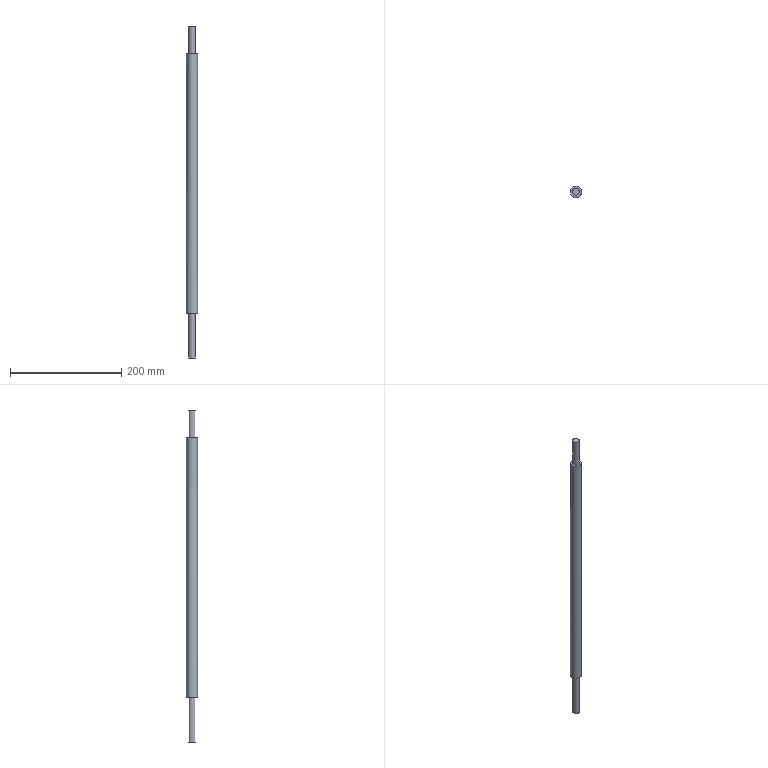Part | STEP file | chuandongzhou | 1 solid | 7 faces | box 20 x 20 x 596.6 mm | volume 161289 mm3 | plane 4 | cylinder 3 | commonest cylinder face diameters 12 x2 20 x1
STEP:
#1=CARTESIAN_POINT('',(0.,0.,0.));
#2=DIRECTION('',(0.,0.,1.));
#3=DIRECTION('',(1.,0.,0.));
#4=AXIS2_PLACEMENT_3D('',#1,#2,#3);
#5=CARTESIAN_POINT('',(-1061.818,-832.005,-786.336));
#6=VERTEX_POINT('',#5);
#7=CARTESIAN_POINT('',(-1061.818,-842.005,-786.336));
#8=DIRECTION('',(0.,0.,1.));
#9=DIRECTION('',(0.,1.,0.));
#10=AXIS2_PLACEMENT_3D('',#7,#8,#9);
#11=CIRCLE('',#10,10.);
#12=CARTESIAN_POINT('',(-1061.818,-842.005,-95.741));
#13=DIRECTION('',(0.,0.,-1.));
#14=DIRECTION('',(0.,1.,0.));
#15=AXIS2_PLACEMENT_3D('',#12,#13,#14);
#16=CYLINDRICAL_SURFACE('',#15,10.);
#17=CARTESIAN_POINT('',(6.283,690.595));
#18=DIRECTION('',(-1.,0.));
#19=VECTOR('',#18,1.);
#20=LINE('',#17,#19);
#21=(GEOMETRIC_REPRESENTATION_CONTEXT(2)PARAMETRIC_REPRESENTATION_CONTEXT()REPRESENTATION_CONTEXT('',''));
#22=DEFINITIONAL_REPRESENTATION('',(#20),#21);
#23=PCURVE('',#16,#22);
#24=CARTESIAN_POINT('',(-1061.818,-842.005,-786.336));
#25=DIRECTION('',(0.,0.,-1.));
#26=DIRECTION('',(0.,1.,0.));
#27=AXIS2_PLACEMENT_3D('',#24,#25,#26);
#28=PLANE('',#27);
#29=CARTESIAN_POINT('',(10.,0.));
#30=CARTESIAN_POINT('',(10.,-17.321));
#31=CARTESIAN_POINT('',(-5.,-8.66));
#32=CARTESIAN_POINT('',(-20.,0.));
#33=CARTESIAN_POINT('',(-5.,8.66));
#34=CARTESIAN_POINT('',(10.,17.321));
#35=CARTESIAN_POINT('',(10.,0.));
#36=(BOUNDED_CURVE()B_SPLINE_CURVE(2,(#29,#30,#31,#32,#33,#34,#35),.UNSPECIFIED.,.T.,.F.)B_SPLINE_CURVE_WITH_KNOTS((1,2,2,2,2,1),(-2.094,0.,2.094,4.189,6.283,8.378),.UNSPECIFIED.)CURVE()GEOMETRIC_REPRESENTATION_ITEM()RATIONAL_B_SPLINE_CURVE((1.,0.5,1.,0.5,1.,0.5,1.))REPRESENTATION_ITEM(''));
#37=(GEOMETRIC_REPRESENTATION_CONTEXT(2)PARAMETRIC_REPRESENTATION_CONTEXT()REPRESENTATION_CONTEXT('',''));
#38=DEFINITIONAL_REPRESENTATION('',(#36),#37);
#39=PCURVE('',#28,#38);
#40=SURFACE_CURVE('',#11,(#23,#39),.PCURVE_S1.);
#41=EDGE_CURVE('',#6,#6,#40,.T.);
#42=ORIENTED_EDGE('',*,*,#41,.T.);
#43=CARTESIAN_POINT('',(-1061.818,-832.005,-319.736));
#44=VERTEX_POINT('',#43);
#45=CARTESIAN_POINT('',(-1061.818,-832.005,-319.736));
#46=CARTESIAN_POINT('',(-1061.818,-832.005,-786.336));
#47=B_SPLINE_CURVE_WITH_KNOTS('',1,(#45,#46),.UNSPECIFIED.,.F.,.F.,(2,2),(223.995,690.595),.PIECEWISE_BEZIER_KNOTS.);
#48=CARTESIAN_POINT('',(0.,0.));
#49=DIRECTION('',(0.,1.));
#50=VECTOR('',#49,1.);
#51=LINE('',#48,#50);
#52=(GEOMETRIC_REPRESENTATION_CONTEXT(2)PARAMETRIC_REPRESENTATION_CONTEXT()REPRESENTATION_CONTEXT('',''));
#53=DEFINITIONAL_REPRESENTATION('',(#51),#52);
#54=PCURVE('',#16,#53);
#55=CARTESIAN_POINT('',(6.283,0.));
#56=DIRECTION('',(0.,1.));
#57=VECTOR('',#56,1.);
#58=LINE('',#55,#57);
#59=(GEOMETRIC_REPRESENTATION_CONTEXT(2)PARAMETRIC_REPRESENTATION_CONTEXT()REPRESENTATION_CONTEXT('',''));
#60=DEFINITIONAL_REPRESENTATION('',(#58),#59);
#61=PCURVE('',#16,#60);
#62=SEAM_CURVE('',#47,(#54,#61),.PCURVE_S1.);
#63=EDGE_CURVE('',#44,#6,#62,.T.);
#64=ORIENTED_EDGE('',*,*,#63,.F.);
#65=CARTESIAN_POINT('',(-1051.818,-842.005,-319.736));
#66=VERTEX_POINT('',#65);
#67=CARTESIAN_POINT('',(-1061.818,-842.005,-319.736));
#68=DIRECTION('',(0.,0.,1.));
#69=DIRECTION('',(1.,0.,0.));
#70=AXIS2_PLACEMENT_3D('',#67,#68,#69);
#71=CIRCLE('',#70,10.);
#72=CARTESIAN_POINT('',(1.571,223.995));
#73=DIRECTION('',(-1.,0.));
#74=VECTOR('',#73,1.);
#75=LINE('',#72,#74);
#76=(GEOMETRIC_REPRESENTATION_CONTEXT(2)PARAMETRIC_REPRESENTATION_CONTEXT()REPRESENTATION_CONTEXT('',''));
#77=DEFINITIONAL_REPRESENTATION('',(#75),#76);
#78=PCURVE('',#16,#77);
#79=CARTESIAN_POINT('',(-1061.818,-842.005,-319.736));
#80=DIRECTION('',(0.,0.,1.));
#81=DIRECTION('',(1.,0.,0.));
#82=AXIS2_PLACEMENT_3D('',#79,#80,#81);
#83=PLANE('',#82);
#84=CARTESIAN_POINT('',(0.,0.));
#85=DIRECTION('',(1.,0.));
#86=AXIS2_PLACEMENT_2D('',#84,#85);
#87=CIRCLE('',#86,10.);
#88=(GEOMETRIC_REPRESENTATION_CONTEXT(2)PARAMETRIC_REPRESENTATION_CONTEXT()REPRESENTATION_CONTEXT('',''));
#89=DEFINITIONAL_REPRESENTATION('',(#87),#88);
#90=PCURVE('',#83,#89);
#91=SURFACE_CURVE('',#71,(#78,#90),.PCURVE_S1.);
#92=EDGE_CURVE('',#66,#44,#91,.T.);
#93=ORIENTED_EDGE('',*,*,#92,.F.);
#94=CARTESIAN_POINT('',(-1061.818,-842.005,-319.736));
#95=DIRECTION('',(0.,0.,1.));
#96=DIRECTION('',(1.,0.,0.));
#97=AXIS2_PLACEMENT_3D('',#94,#95,#96);
#98=CIRCLE('',#97,10.);
#99=CARTESIAN_POINT('',(7.854,223.995));
#100=DIRECTION('',(-1.,0.));
#101=VECTOR('',#100,1.);
#102=LINE('',#99,#101);
#103=(GEOMETRIC_REPRESENTATION_CONTEXT(2)PARAMETRIC_REPRESENTATION_CONTEXT()REPRESENTATION_CONTEXT('',''));
#104=DEFINITIONAL_REPRESENTATION('',(#102),#103);
#105=PCURVE('',#16,#104);
#106=CARTESIAN_POINT('',(0.,0.));
#107=DIRECTION('',(1.,0.));
#108=AXIS2_PLACEMENT_2D('',#106,#107);
#109=CIRCLE('',#108,10.);
#110=(GEOMETRIC_REPRESENTATION_CONTEXT(2)PARAMETRIC_REPRESENTATION_CONTEXT()REPRESENTATION_CONTEXT('',''));
#111=DEFINITIONAL_REPRESENTATION('',(#109),#110);
#112=PCURVE('',#83,#111);
#113=SURFACE_CURVE('',#98,(#105,#112),.PCURVE_S1.);
#114=EDGE_CURVE('',#44,#66,#113,.T.);
#115=ORIENTED_EDGE('',*,*,#114,.F.);
#116=ORIENTED_EDGE('',*,*,#63,.T.);
#117=EDGE_LOOP('',(#42,#64,#93,#115,#116));
#118=FACE_BOUND('',#117,.T.);
#119=ADVANCED_FACE('',(#118),#16,.T.);
#120=ORIENTED_EDGE('',*,*,#41,.F.);
#121=EDGE_LOOP('',(#120));
#122=FACE_BOUND('',#121,.T.);
#123=CARTESIAN_POINT('',(-1055.818,-842.005,-786.336));
#124=VERTEX_POINT('',#123);
#125=CARTESIAN_POINT('',(-1061.818,-842.005,-786.336));
#126=DIRECTION('',(0.,0.,1.));
#127=DIRECTION('',(1.,0.,0.));
#128=AXIS2_PLACEMENT_3D('',#125,#126,#127);
#129=CIRCLE('',#128,6.);
#130=CARTESIAN_POINT('',(0.,6.));
#131=CARTESIAN_POINT('',(10.392,6.));
#132=CARTESIAN_POINT('',(5.196,-3.));
#133=CARTESIAN_POINT('',(0.,-12.));
#134=CARTESIAN_POINT('',(-5.196,-3.));
#135=CARTESIAN_POINT('',(-10.392,6.));
#136=CARTESIAN_POINT('',(0.,6.));
#137=(BOUNDED_CURVE()B_SPLINE_CURVE(2,(#130,#131,#132,#133,#134,#135,#136),.UNSPECIFIED.,.T.,.F.)B_SPLINE_CURVE_WITH_KNOTS((1,2,2,2,2,1),(-2.094,0.,2.094,4.189,6.283,8.378),.UNSPECIFIED.)CURVE()GEOMETRIC_REPRESENTATION_ITEM()RATIONAL_B_SPLINE_CURVE((1.,0.5,1.,0.5,1.,0.5,1.))REPRESENTATION_ITEM(''));
#138=(GEOMETRIC_REPRESENTATION_CONTEXT(2)PARAMETRIC_REPRESENTATION_CONTEXT()REPRESENTATION_CONTEXT('',''));
#139=DEFINITIONAL_REPRESENTATION('',(#137),#138);
#140=PCURVE('',#28,#139);
#141=CARTESIAN_POINT('',(-1061.818,-842.005,-866.336));
#142=DIRECTION('',(0.,0.,1.));
#143=DIRECTION('',(1.,0.,0.));
#144=AXIS2_PLACEMENT_3D('',#141,#142,#143);
#145=CYLINDRICAL_SURFACE('',#144,6.);
#146=CARTESIAN_POINT('',(0.,80.));
#147=DIRECTION('',(1.,0.));
#148=VECTOR('',#147,1.);
#149=LINE('',#146,#148);
#150=(GEOMETRIC_REPRESENTATION_CONTEXT(2)PARAMETRIC_REPRESENTATION_CONTEXT()REPRESENTATION_CONTEXT('',''));
#151=DEFINITIONAL_REPRESENTATION('',(#149),#150);
#152=PCURVE('',#145,#151);
#153=SURFACE_CURVE('',#129,(#140,#152),.PCURVE_S1.);
#154=EDGE_CURVE('',#124,#124,#153,.T.);
#155=ORIENTED_EDGE('',*,*,#154,.T.);
#156=EDGE_LOOP('',(#155));
#157=FACE_BOUND('',#156,.T.);
#158=ADVANCED_FACE('',(#122,#157),#28,.T.);
#159=CARTESIAN_POINT('',(-1055.818,-842.005,-866.336));
#160=VERTEX_POINT('',#159);
#161=CARTESIAN_POINT('',(-1061.818,-842.005,-866.336));
#162=DIRECTION('',(0.,0.,1.));
#163=DIRECTION('',(1.,0.,0.));
#164=AXIS2_PLACEMENT_3D('',#161,#162,#163);
#165=CIRCLE('',#164,6.);
#166=CARTESIAN_POINT('',(0.,0.));
#167=DIRECTION('',(1.,0.));
#168=VECTOR('',#167,1.);
#169=LINE('',#166,#168);
#170=(GEOMETRIC_REPRESENTATION_CONTEXT(2)PARAMETRIC_REPRESENTATION_CONTEXT()REPRESENTATION_CONTEXT('',''));
#171=DEFINITIONAL_REPRESENTATION('',(#169),#170);
#172=PCURVE('',#145,#171);
#173=CARTESIAN_POINT('',(-1061.818,-842.005,-866.336));
#174=DIRECTION('',(0.,0.,1.));
#175=DIRECTION('',(1.,0.,0.));
#176=AXIS2_PLACEMENT_3D('',#173,#174,#175);
#177=PLANE('',#176);
#178=CARTESIAN_POINT('',(0.,0.));
#179=DIRECTION('',(1.,0.));
#180=AXIS2_PLACEMENT_2D('',#178,#179);
#181=CIRCLE('',#180,6.);
#182=(GEOMETRIC_REPRESENTATION_CONTEXT(2)PARAMETRIC_REPRESENTATION_CONTEXT()REPRESENTATION_CONTEXT('',''));
#183=DEFINITIONAL_REPRESENTATION('',(#181),#182);
#184=PCURVE('',#177,#183);
#185=SURFACE_CURVE('',#165,(#172,#184),.PCURVE_S1.);
#186=EDGE_CURVE('',#160,#160,#185,.T.);
#187=ORIENTED_EDGE('',*,*,#186,.T.);
#188=CARTESIAN_POINT('',(-1055.818,-842.005,-866.336));
#189=CARTESIAN_POINT('',(-1055.818,-842.005,-786.336));
#190=B_SPLINE_CURVE_WITH_KNOTS('',1,(#188,#189),.UNSPECIFIED.,.F.,.F.,(2,2),(0.,80.),.PIECEWISE_BEZIER_KNOTS.);
#191=CARTESIAN_POINT('',(6.283,0.));
#192=DIRECTION('',(0.,1.));
#193=VECTOR('',#192,1.);
#194=LINE('',#191,#193);
#195=(GEOMETRIC_REPRESENTATION_CONTEXT(2)PARAMETRIC_REPRESENTATION_CONTEXT()REPRESENTATION_CONTEXT('',''));
#196=DEFINITIONAL_REPRESENTATION('',(#194),#195);
#197=PCURVE('',#145,#196);
#198=CARTESIAN_POINT('',(0.,0.));
#199=DIRECTION('',(0.,1.));
#200=VECTOR('',#199,1.);
#201=LINE('',#198,#200);
#202=(GEOMETRIC_REPRESENTATION_CONTEXT(2)PARAMETRIC_REPRESENTATION_CONTEXT()REPRESENTATION_CONTEXT('',''));
#203=DEFINITIONAL_REPRESENTATION('',(#201),#202);
#204=PCURVE('',#145,#203);
#205=SEAM_CURVE('',#190,(#197,#204),.PCURVE_S1.);
#206=EDGE_CURVE('',#160,#124,#205,.T.);
#207=ORIENTED_EDGE('',*,*,#206,.T.);
#208=ORIENTED_EDGE('',*,*,#154,.F.);
#209=ORIENTED_EDGE('',*,*,#206,.F.);
#210=EDGE_LOOP('',(#187,#207,#208,#209));
#211=FACE_BOUND('',#210,.T.);
#212=ADVANCED_FACE('',(#211),#145,.T.);
#213=ORIENTED_EDGE('',*,*,#186,.F.);
#214=EDGE_LOOP('',(#213));
#215=FACE_BOUND('',#214,.T.);
#216=ADVANCED_FACE('',(#215),#177,.F.);
#217=CARTESIAN_POINT('',(-1055.818,-842.005,-319.736));
#218=VERTEX_POINT('',#217);
#219=CARTESIAN_POINT('',(-1061.818,-842.005,-319.736));
#220=DIRECTION('',(0.,0.,1.));
#221=DIRECTION('',(1.,0.,0.));
#222=AXIS2_PLACEMENT_3D('',#219,#220,#221);
#223=CIRCLE('',#222,6.);
#224=CARTESIAN_POINT('',(0.,0.));
#225=DIRECTION('',(1.,0.));
#226=AXIS2_PLACEMENT_2D('',#224,#225);
#227=CIRCLE('',#226,6.);
#228=(GEOMETRIC_REPRESENTATION_CONTEXT(2)PARAMETRIC_REPRESENTATION_CONTEXT()REPRESENTATION_CONTEXT('',''));
#229=DEFINITIONAL_REPRESENTATION('',(#227),#228);
#230=PCURVE('',#83,#229);
#231=CARTESIAN_POINT('',(-1061.818,-842.005,-269.736));
#232=DIRECTION('',(0.,0.,-1.));
#233=DIRECTION('',(-1.,0.,0.));
#234=AXIS2_PLACEMENT_3D('',#231,#232,#233);
#235=CYLINDRICAL_SURFACE('',#234,6.);
#236=CARTESIAN_POINT('',(9.425,50.));
#237=DIRECTION('',(-1.,0.));
#238=VECTOR('',#237,1.);
#239=LINE('',#236,#238);
#240=(GEOMETRIC_REPRESENTATION_CONTEXT(2)PARAMETRIC_REPRESENTATION_CONTEXT()REPRESENTATION_CONTEXT('',''));
#241=DEFINITIONAL_REPRESENTATION('',(#239),#240);
#242=PCURVE('',#235,#241);
#243=SURFACE_CURVE('',#223,(#230,#242),.PCURVE_S1.);
#244=EDGE_CURVE('',#218,#218,#243,.T.);
#245=ORIENTED_EDGE('',*,*,#244,.F.);
#246=EDGE_LOOP('',(#245));
#247=FACE_BOUND('',#246,.T.);
#248=ORIENTED_EDGE('',*,*,#92,.T.);
#249=ORIENTED_EDGE('',*,*,#114,.T.);
#250=EDGE_LOOP('',(#248,#249));
#251=FACE_BOUND('',#250,.T.);
#252=ADVANCED_FACE('',(#247,#251),#83,.T.);
#253=CARTESIAN_POINT('',(-1055.818,-842.005,-269.736));
#254=VERTEX_POINT('',#253);
#255=CARTESIAN_POINT('',(-1061.818,-842.005,-269.736));
#256=DIRECTION('',(0.,0.,1.));
#257=DIRECTION('',(1.,0.,0.));
#258=AXIS2_PLACEMENT_3D('',#255,#256,#257);
#259=CIRCLE('',#258,6.);
#260=CARTESIAN_POINT('',(9.425,0.));
#261=DIRECTION('',(-1.,0.));
#262=VECTOR('',#261,1.);
#263=LINE('',#260,#262);
#264=(GEOMETRIC_REPRESENTATION_CONTEXT(2)PARAMETRIC_REPRESENTATION_CONTEXT()REPRESENTATION_CONTEXT('',''));
#265=DEFINITIONAL_REPRESENTATION('',(#263),#264);
#266=PCURVE('',#235,#265);
#267=CARTESIAN_POINT('',(-1061.818,-842.005,-269.736));
#268=DIRECTION('',(0.,0.,1.));
#269=DIRECTION('',(1.,0.,0.));
#270=AXIS2_PLACEMENT_3D('',#267,#268,#269);
#271=PLANE('',#270);
#272=CARTESIAN_POINT('',(0.,0.));
#273=DIRECTION('',(1.,0.));
#274=AXIS2_PLACEMENT_2D('',#272,#273);
#275=CIRCLE('',#274,6.);
#276=(GEOMETRIC_REPRESENTATION_CONTEXT(2)PARAMETRIC_REPRESENTATION_CONTEXT()REPRESENTATION_CONTEXT('',''));
#277=DEFINITIONAL_REPRESENTATION('',(#275),#276);
#278=PCURVE('',#271,#277);
#279=SURFACE_CURVE('',#259,(#266,#278),.PCURVE_S1.);
#280=EDGE_CURVE('',#254,#254,#279,.T.);
#281=ORIENTED_EDGE('',*,*,#280,.F.);
#282=CARTESIAN_POINT('',(-1055.818,-842.005,-269.736));
#283=CARTESIAN_POINT('',(-1055.818,-842.005,-319.736));
#284=B_SPLINE_CURVE_WITH_KNOTS('',1,(#282,#283),.UNSPECIFIED.,.F.,.F.,(2,2),(0.,50.),.PIECEWISE_BEZIER_KNOTS.);
#285=CARTESIAN_POINT('',(9.425,0.));
#286=DIRECTION('',(0.,1.));
#287=VECTOR('',#286,1.);
#288=LINE('',#285,#287);
#289=(GEOMETRIC_REPRESENTATION_CONTEXT(2)PARAMETRIC_REPRESENTATION_CONTEXT()REPRESENTATION_CONTEXT('',''));
#290=DEFINITIONAL_REPRESENTATION('',(#288),#289);
#291=PCURVE('',#235,#290);
#292=CARTESIAN_POINT('',(3.142,0.));
#293=DIRECTION('',(0.,1.));
#294=VECTOR('',#293,1.);
#295=LINE('',#292,#294);
#296=(GEOMETRIC_REPRESENTATION_CONTEXT(2)PARAMETRIC_REPRESENTATION_CONTEXT()REPRESENTATION_CONTEXT('',''));
#297=DEFINITIONAL_REPRESENTATION('',(#295),#296);
#298=PCURVE('',#235,#297);
#299=SEAM_CURVE('',#284,(#291,#298),.PCURVE_S1.);
#300=EDGE_CURVE('',#254,#218,#299,.T.);
#301=ORIENTED_EDGE('',*,*,#300,.T.);
#302=ORIENTED_EDGE('',*,*,#244,.T.);
#303=ORIENTED_EDGE('',*,*,#300,.F.);
#304=EDGE_LOOP('',(#281,#301,#302,#303));
#305=FACE_BOUND('',#304,.T.);
#306=ADVANCED_FACE('',(#305),#235,.T.);
#307=ORIENTED_EDGE('',*,*,#280,.T.);
#308=EDGE_LOOP('',(#307));
#309=FACE_BOUND('',#308,.T.);
#310=ADVANCED_FACE('',(#309),#271,.T.);
#311=CLOSED_SHELL('',(#119,#158,#212,#216,#252,#306,#310));
#312=MANIFOLD_SOLID_BREP('',#311);
#313=(LENGTH_UNIT()NAMED_UNIT(*)SI_UNIT(.MILLI.,.METRE.));
#314=UNCERTAINTY_MEASURE_WITH_UNIT(LENGTH_MEASURE(0.000005),#313,'','');
#315=(NAMED_UNIT(*)PLANE_ANGLE_UNIT()SI_UNIT($,.RADIAN.));
#316=(NAMED_UNIT(*)SI_UNIT($,.STERADIAN.)SOLID_ANGLE_UNIT());
#317=(GEOMETRIC_REPRESENTATION_CONTEXT(3)GLOBAL_UNCERTAINTY_ASSIGNED_CONTEXT((#314))GLOBAL_UNIT_ASSIGNED_CONTEXT((#313,#315,#316))REPRESENTATION_CONTEXT('',''));
#318=ADVANCED_BREP_SHAPE_REPRESENTATION('',(#4,#312),#317);